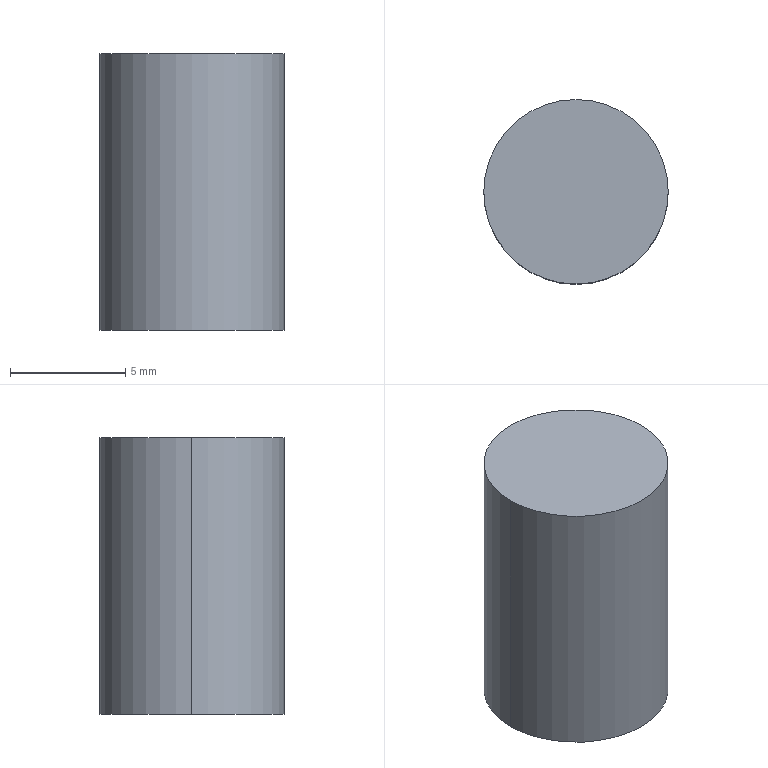Part | SolidWorks | features Extrusion 1 | 1 solid | 4 faces | box 8 x 8 x 12 mm | volume 603.186 mm3 | cylinder 2 | plane 2 | commonest cylinder face diameters 8 x2
STEP:
#1=CARTESIAN_POINT('',(4.,0.,-6.));
#2=VERTEX_POINT('',#1);
#3=CARTESIAN_POINT('',(-4.,0.,-6.));
#4=VERTEX_POINT('',#3);
#5=CARTESIAN_POINT('',(0.,0.,-6.));
#6=DIRECTION('',(0.,0.,1.));
#7=DIRECTION('',(1.,0.,0.));
#8=AXIS2_PLACEMENT_3D('',#5,#6,#7);
#9=CIRCLE('',#8,4.);
#10=EDGE_CURVE('',#2,#4,#9,.T.);
#11=ORIENTED_EDGE('',*,*,#10,.T.);
#12=CARTESIAN_POINT('',(-4.,0.,6.));
#13=VERTEX_POINT('',#12);
#14=CARTESIAN_POINT('',(-4.,0.,-6.));
#15=DIRECTION('',(0.,0.,1.));
#16=VECTOR('',#15,1000.);
#17=LINE('',#14,#16);
#18=EDGE_CURVE('',#4,#13,#17,.T.);
#19=ORIENTED_EDGE('',*,*,#18,.T.);
#20=CARTESIAN_POINT('',(4.,0.,6.));
#21=VERTEX_POINT('',#20);
#22=CARTESIAN_POINT('',(0.,0.,6.));
#23=DIRECTION('',(0.,0.,1.));
#24=DIRECTION('',(1.,0.,0.));
#25=AXIS2_PLACEMENT_3D('',#22,#23,#24);
#26=CIRCLE('',#25,4.);
#27=EDGE_CURVE('',#21,#13,#26,.T.);
#28=ORIENTED_EDGE('',*,*,#27,.F.);
#29=CARTESIAN_POINT('',(4.,0.,-6.));
#30=DIRECTION('',(0.,0.,1.));
#31=VECTOR('',#30,1000.);
#32=LINE('',#29,#31);
#33=EDGE_CURVE('',#2,#21,#32,.T.);
#34=ORIENTED_EDGE('',*,*,#33,.F.);
#35=EDGE_LOOP('',(#11,#19,#28,#34));
#36=FACE_OUTER_BOUND('',#35,.T.);
#37=CARTESIAN_POINT('',(0.,0.,-6.));
#38=DIRECTION('',(0.,0.,1.));
#39=DIRECTION('',(1.,0.,0.));
#40=AXIS2_PLACEMENT_3D('',#37,#38,#39);
#41=CYLINDRICAL_SURFACE('',#40,4.);
#42=ADVANCED_FACE('',(#36),#41,.T.);
#43=ORIENTED_EDGE('',*,*,#18,.F.);
#44=CARTESIAN_POINT('',(0.,0.,-6.));
#45=DIRECTION('',(0.,0.,1.));
#46=DIRECTION('',(1.,0.,0.));
#47=AXIS2_PLACEMENT_3D('',#44,#45,#46);
#48=CIRCLE('',#47,4.);
#49=EDGE_CURVE('',#4,#2,#48,.T.);
#50=ORIENTED_EDGE('',*,*,#49,.T.);
#51=ORIENTED_EDGE('',*,*,#33,.T.);
#52=CARTESIAN_POINT('',(0.,0.,6.));
#53=DIRECTION('',(0.,0.,1.));
#54=DIRECTION('',(1.,0.,0.));
#55=AXIS2_PLACEMENT_3D('',#52,#53,#54);
#56=CIRCLE('',#55,4.);
#57=EDGE_CURVE('',#13,#21,#56,.T.);
#58=ORIENTED_EDGE('',*,*,#57,.F.);
#59=EDGE_LOOP('',(#43,#50,#51,#58));
#60=FACE_OUTER_BOUND('',#59,.T.);
#61=CARTESIAN_POINT('',(0.,0.,-6.));
#62=DIRECTION('',(0.,0.,1.));
#63=DIRECTION('',(1.,0.,0.));
#64=AXIS2_PLACEMENT_3D('',#61,#62,#63);
#65=CYLINDRICAL_SURFACE('',#64,4.);
#66=ADVANCED_FACE('',(#60),#65,.T.);
#67=ORIENTED_EDGE('',*,*,#10,.F.);
#68=ORIENTED_EDGE('',*,*,#49,.F.);
#69=EDGE_LOOP('',(#67,#68));
#70=FACE_OUTER_BOUND('',#69,.T.);
#71=CARTESIAN_POINT('',(0.,0.,-6.));
#72=DIRECTION('',(0.,0.,1.));
#73=DIRECTION('',(1.,0.,0.));
#74=AXIS2_PLACEMENT_3D('',#71,#72,#73);
#75=PLANE('',#74);
#76=ADVANCED_FACE('',(#70),#75,.F.);
#77=ORIENTED_EDGE('',*,*,#27,.T.);
#78=ORIENTED_EDGE('',*,*,#57,.T.);
#79=EDGE_LOOP('',(#77,#78));
#80=FACE_OUTER_BOUND('',#79,.T.);
#81=CARTESIAN_POINT('',(0.,0.,6.));
#82=DIRECTION('',(0.,0.,1.));
#83=DIRECTION('',(1.,0.,0.));
#84=AXIS2_PLACEMENT_3D('',#81,#82,#83);
#85=PLANE('',#84);
#86=ADVANCED_FACE('',(#80),#85,.T.);
#87=CLOSED_SHELL('',(#42,#66,#76,#86));
#88=MANIFOLD_SOLID_BREP('',#87);
#89=CARTESIAN_POINT('',(0.,0.,0.));
#90=DIRECTION('',(0.,0.,1.));
#91=DIRECTION('',(1.,0.,0.));
#92=AXIS2_PLACEMENT_3D('',#89,#90,#91);
#93=(LENGTH_UNIT()NAMED_UNIT(*)SI_UNIT(.MILLI.,.METRE.));
#94=UNCERTAINTY_MEASURE_WITH_UNIT(LENGTH_MEASURE(0.00001),#93,'','');
#95=(NAMED_UNIT(*)PLANE_ANGLE_UNIT()SI_UNIT($,.RADIAN.));
#96=(NAMED_UNIT(*)SI_UNIT($,.STERADIAN.)SOLID_ANGLE_UNIT());
#97=(GEOMETRIC_REPRESENTATION_CONTEXT(3)GLOBAL_UNCERTAINTY_ASSIGNED_CONTEXT((#94))GLOBAL_UNIT_ASSIGNED_CONTEXT((#93,#95,#96))REPRESENTATION_CONTEXT('',''));
#98=ADVANCED_BREP_SHAPE_REPRESENTATION('',(#88,#92),#97);